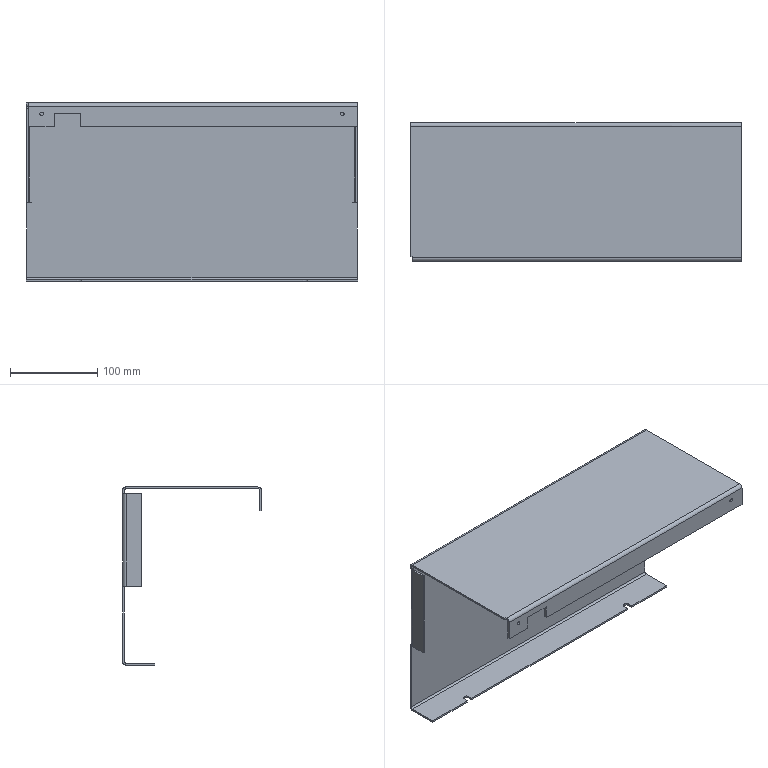Part | NX | features 5003_227_Cover 2 | 1 solid | 86 faces | box 379.277 x 159 x 204 mm | volume 322904 mm3 | plane 68 | cylinder 14 | spline 4 | commonest cylinder face diameters 4 x5 8 x5 4.134 x2 7 x2